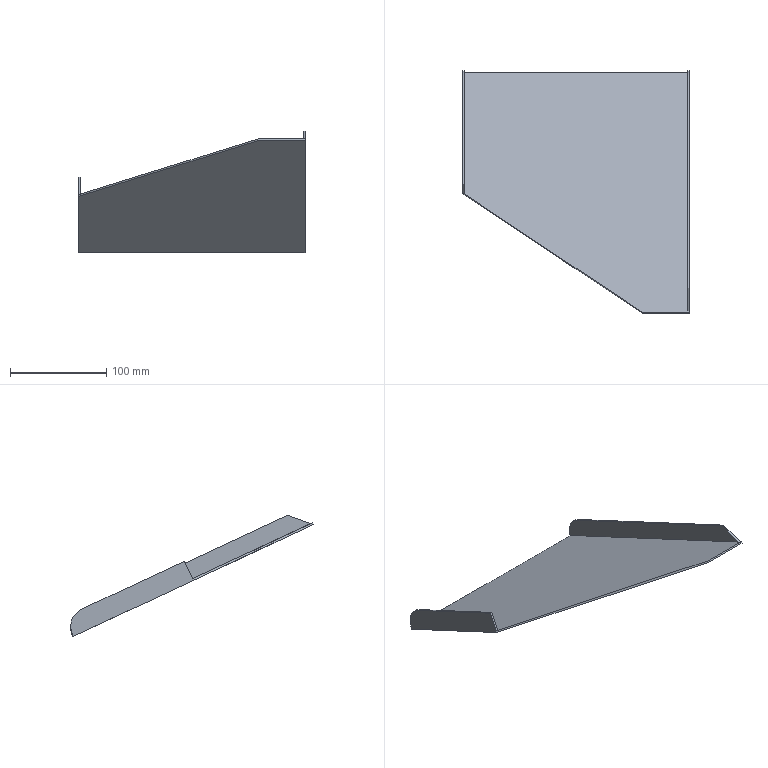Part | NX | features solid 2 | 1 solid | 15 faces | box 235.691 x 251.874 x 126.251 mm | volume 118871 mm3 | plane 13 | cylinder 2 | commonest cylinder face diameters 40 x2
STEP:
#1=CARTESIAN_POINT('',(530.986,470.,-185.082));
#2=VERTEX_POINT('',#1);
#3=CARTESIAN_POINT('',(344.309,594.452,-243.115));
#4=VERTEX_POINT('',#3);
#5=CARTESIAN_POINT('',(383.264,568.481,-231.004));
#6=DIRECTION('',(-0.8055,0.537,-0.2504));
#7=VECTOR('',#6,1000.);
#8=LINE('',#5,#7);
#9=EDGE_CURVE('',#2,#4,#8,.T.);
#10=ORIENTED_EDGE('',*,*,#9,.F.);
#11=CARTESIAN_POINT('',(530.986,470.845,-183.269));
#12=VERTEX_POINT('',#11);
#13=CARTESIAN_POINT('',(530.986,470.845,-183.269));
#14=DIRECTION('',(0.,-0.4226,-0.9063));
#15=VECTOR('',#14,1000.);
#16=LINE('',#13,#15);
#17=EDGE_CURVE('',#12,#2,#16,.T.);
#18=ORIENTED_EDGE('',*,*,#17,.F.);
#19=CARTESIAN_POINT('',(344.309,595.297,-241.302));
#20=VERTEX_POINT('',#19);
#21=CARTESIAN_POINT('',(383.264,569.326,-229.192));
#22=DIRECTION('',(-0.8055,0.537,-0.2504));
#23=VECTOR('',#22,1000.);
#24=LINE('',#21,#23);
#25=EDGE_CURVE('',#12,#20,#24,.T.);
#26=ORIENTED_EDGE('',*,*,#25,.T.);
#27=CARTESIAN_POINT('',(344.309,595.297,-241.302));
#28=DIRECTION('',(0.,-0.4226,-0.9063));
#29=VECTOR('',#28,1000.);
#30=LINE('',#27,#29);
#31=EDGE_CURVE('',#20,#4,#30,.T.);
#32=ORIENTED_EDGE('',*,*,#31,.T.);
#33=EDGE_LOOP('',(#10,#18,#26,#32));
#34=FACE_BOUND('',#33,.T.);
#35=CARTESIAN_POINT('',(383.264,569.326,-229.192));
#36=DIRECTION('',(-0.5925,-0.7301,0.3404));
#37=DIRECTION('',(0.7764,-0.6302,0.));
#38=AXIS2_PLACEMENT_3D('',#35,#36,#37);
#39=PLANE('',#38);
#40=ADVANCED_FACE('',(#34),#39,.T.);
#41=CARTESIAN_POINT('',(580.,470.,-185.082));
#42=VERTEX_POINT('',#41);
#43=CARTESIAN_POINT('',(570.,470.,-185.082));
#44=DIRECTION('',(-1.,0.,0.));
#45=VECTOR('',#44,1000.);
#46=LINE('',#43,#45);
#47=EDGE_CURVE('',#2,#42,#46,.F.);
#48=ORIENTED_EDGE('',*,*,#47,.T.);
#49=CARTESIAN_POINT('',(580.,470.845,-183.269));
#50=VERTEX_POINT('',#49);
#51=CARTESIAN_POINT('',(580.,470.845,-183.269));
#52=DIRECTION('',(0.,-0.4226,-0.9063));
#53=VECTOR('',#52,1000.);
#54=LINE('',#51,#53);
#55=EDGE_CURVE('',#50,#42,#54,.T.);
#56=ORIENTED_EDGE('',*,*,#55,.F.);
#57=CARTESIAN_POINT('',(570.,470.845,-183.269));
#58=DIRECTION('',(-1.,0.,0.));
#59=VECTOR('',#58,1000.);
#60=LINE('',#57,#59);
#61=EDGE_CURVE('',#12,#50,#60,.F.);
#62=ORIENTED_EDGE('',*,*,#61,.F.);
#63=ORIENTED_EDGE('',*,*,#17,.T.);
#64=EDGE_LOOP('',(#48,#56,#62,#63));
#65=FACE_BOUND('',#64,.T.);
#66=CARTESIAN_POINT('',(570.,470.845,-183.269));
#67=DIRECTION('',(0.,0.9063,-0.4226));
#68=DIRECTION('',(0.,0.4226,0.9063));
#69=AXIS2_PLACEMENT_3D('',#66,#67,#68);
#70=PLANE('',#69);
#71=ADVANCED_FACE('',(#65),#70,.F.);
#72=ORIENTED_EDGE('',*,*,#55,.T.);
#73=CARTESIAN_POINT('',(580.,720.,-301.659));
#74=VERTEX_POINT('',#73);
#75=CARTESIAN_POINT('',(580.,581.797,-237.214));
#76=DIRECTION('',(0.,-0.9063,0.4226));
#77=VECTOR('',#76,1000.);
#78=LINE('',#75,#77);
#79=EDGE_CURVE('',#74,#42,#78,.T.);
#80=ORIENTED_EDGE('',*,*,#79,.F.);
#81=CARTESIAN_POINT('',(580.,710.326,-275.08));
#82=VERTEX_POINT('',#81);
#83=CARTESIAN_POINT('',(580.,701.874,-293.206));
#84=DIRECTION('',(1.,0.,0.));
#85=DIRECTION('',(0.,0.,-1.));
#86=AXIS2_PLACEMENT_3D('',#83,#84,#85);
#87=CIRCLE('',#86,20.);
#88=EDGE_CURVE('',#74,#82,#87,.T.);
#89=ORIENTED_EDGE('',*,*,#88,.T.);
#90=CARTESIAN_POINT('',(580.,496.579,-175.408));
#91=VERTEX_POINT('',#90);
#92=CARTESIAN_POINT('',(580.,728.452,-283.533));
#93=DIRECTION('',(0.,-0.9063,0.4226));
#94=VECTOR('',#93,1000.);
#95=LINE('',#92,#94);
#96=EDGE_CURVE('',#82,#91,#95,.T.);
#97=ORIENTED_EDGE('',*,*,#96,.T.);
#98=CARTESIAN_POINT('',(580.,472.658,-184.114));
#99=VERTEX_POINT('',#98);
#100=CARTESIAN_POINT('',(580.,553.294,-154.765));
#101=DIRECTION('',(0.,-0.9397,-0.342));
#102=VECTOR('',#101,1000.);
#103=LINE('',#100,#102);
#104=EDGE_CURVE('',#91,#99,#103,.T.);
#105=ORIENTED_EDGE('',*,*,#104,.T.);
#106=CARTESIAN_POINT('',(580.,582.643,-235.401));
#107=DIRECTION('',(0.,-0.9063,0.4226));
#108=VECTOR('',#107,1000.);
#109=LINE('',#106,#108);
#110=EDGE_CURVE('',#99,#50,#109,.T.);
#111=ORIENTED_EDGE('',*,*,#110,.T.);
#112=EDGE_LOOP('',(#72,#80,#89,#97,#105,#111));
#113=FACE_BOUND('',#112,.T.);
#114=CARTESIAN_POINT('',(580.,582.643,-235.401));
#115=DIRECTION('',(1.,0.,0.));
#116=DIRECTION('',(0.,0.,-1.));
#117=AXIS2_PLACEMENT_3D('',#114,#115,#116);
#118=PLANE('',#117);
#119=ADVANCED_FACE('',(#113),#118,.T.);
#120=CARTESIAN_POINT('',(578.,720.,-301.659));
#121=VERTEX_POINT('',#120);
#122=CARTESIAN_POINT('',(578.,720.,-299.452));
#123=VERTEX_POINT('',#122);
#124=CARTESIAN_POINT('',(578.,720.,-430.));
#125=DIRECTION('',(0.,0.,-1.));
#126=VECTOR('',#125,1000.);
#127=LINE('',#124,#126);
#128=EDGE_CURVE('',#121,#123,#127,.F.);
#129=ORIENTED_EDGE('',*,*,#128,.F.);
#130=CARTESIAN_POINT('',(344.309,720.,-301.659));
#131=VERTEX_POINT('',#130);
#132=CARTESIAN_POINT('',(570.,720.,-301.659));
#133=DIRECTION('',(-1.,0.,0.));
#134=VECTOR('',#133,1000.);
#135=LINE('',#132,#134);
#136=EDGE_CURVE('',#131,#121,#135,.F.);
#137=ORIENTED_EDGE('',*,*,#136,.F.);
#138=CARTESIAN_POINT('',(344.309,720.,-299.452));
#139=VERTEX_POINT('',#138);
#140=CARTESIAN_POINT('',(344.309,720.,-430.));
#141=DIRECTION('',(0.,0.,1.));
#142=VECTOR('',#141,1000.);
#143=LINE('',#140,#142);
#144=EDGE_CURVE('',#139,#131,#143,.F.);
#145=ORIENTED_EDGE('',*,*,#144,.F.);
#146=CARTESIAN_POINT('',(346.309,720.,-299.452));
#147=VERTEX_POINT('',#146);
#148=CARTESIAN_POINT('',(570.,720.,-299.452));
#149=DIRECTION('',(-1.,0.,0.));
#150=VECTOR('',#149,1000.);
#151=LINE('',#148,#150);
#152=EDGE_CURVE('',#139,#147,#151,.F.);
#153=ORIENTED_EDGE('',*,*,#152,.T.);
#154=CARTESIAN_POINT('',(570.,720.,-299.452));
#155=DIRECTION('',(-1.,0.,0.));
#156=VECTOR('',#155,1000.);
#157=LINE('',#154,#156);
#158=EDGE_CURVE('',#147,#123,#157,.F.);
#159=ORIENTED_EDGE('',*,*,#158,.T.);
#160=EDGE_LOOP('',(#129,#137,#145,#153,#159));
#161=FACE_BOUND('',#160,.T.);
#162=CARTESIAN_POINT('',(188.564,720.,-430.));
#163=DIRECTION('',(0.,-1.,0.));
#164=DIRECTION('',(-1.,0.,0.));
#165=AXIS2_PLACEMENT_3D('',#162,#163,#164);
#166=PLANE('',#165);
#167=ADVANCED_FACE('',(#161),#166,.F.);
#168=CARTESIAN_POINT('',(344.309,524.315,-210.409));
#169=DIRECTION('',(0.,-0.9063,0.4226));
#170=VECTOR('',#169,1000.);
#171=LINE('',#168,#170);
#172=EDGE_CURVE('',#131,#4,#171,.T.);
#173=ORIENTED_EDGE('',*,*,#172,.T.);
#174=ORIENTED_EDGE('',*,*,#31,.F.);
#175=CARTESIAN_POINT('',(344.309,603.749,-223.176));
#176=VERTEX_POINT('',#175);
#177=CARTESIAN_POINT('',(344.309,595.297,-241.302));
#178=DIRECTION('',(0.,0.4226,0.9063));
#179=VECTOR('',#178,1000.);
#180=LINE('',#177,#179);
#181=EDGE_CURVE('',#20,#176,#180,.T.);
#182=ORIENTED_EDGE('',*,*,#181,.T.);
#183=CARTESIAN_POINT('',(344.309,710.326,-272.873));
#184=VERTEX_POINT('',#183);
#185=CARTESIAN_POINT('',(344.309,728.452,-281.326));
#186=DIRECTION('',(0.,-0.9063,0.4226));
#187=VECTOR('',#186,1000.);
#188=LINE('',#185,#187);
#189=EDGE_CURVE('',#184,#176,#188,.T.);
#190=ORIENTED_EDGE('',*,*,#189,.F.);
#191=CARTESIAN_POINT('',(344.309,701.874,-291.));
#192=DIRECTION('',(-1.,0.,0.));
#193=DIRECTION('',(0.,-1.,0.));
#194=AXIS2_PLACEMENT_3D('',#191,#192,#193);
#195=CIRCLE('',#194,20.);
#196=EDGE_CURVE('',#184,#139,#195,.T.);
#197=ORIENTED_EDGE('',*,*,#196,.T.);
#198=ORIENTED_EDGE('',*,*,#144,.T.);
#199=EDGE_LOOP('',(#173,#174,#182,#190,#197,#198));
#200=FACE_BOUND('',#199,.T.);
#201=CARTESIAN_POINT('',(344.309,525.16,-208.597));
#202=DIRECTION('',(1.,0.,0.));
#203=DIRECTION('',(0.,1.,0.));
#204=AXIS2_PLACEMENT_3D('',#201,#202,#203);
#205=PLANE('',#204);
#206=ADVANCED_FACE('',(#200),#205,.F.);
#207=CARTESIAN_POINT('',(578.,472.658,-184.114));
#208=VERTEX_POINT('',#207);
#209=CARTESIAN_POINT('',(570.,472.658,-184.114));
#210=DIRECTION('',(-1.,0.,0.));
#211=VECTOR('',#210,1000.);
#212=LINE('',#209,#211);
#213=EDGE_CURVE('',#99,#208,#212,.T.);
#214=ORIENTED_EDGE('',*,*,#213,.T.);
#215=CARTESIAN_POINT('',(578.,582.643,-235.401));
#216=DIRECTION('',(0.,0.9063,-0.4226));
#217=VECTOR('',#216,1000.);
#218=LINE('',#215,#217);
#219=EDGE_CURVE('',#208,#123,#218,.T.);
#220=ORIENTED_EDGE('',*,*,#219,.T.);
#221=ORIENTED_EDGE('',*,*,#158,.F.);
#222=CARTESIAN_POINT('',(346.309,595.297,-241.302));
#223=VERTEX_POINT('',#222);
#224=CARTESIAN_POINT('',(346.309,720.,-299.452));
#225=DIRECTION('',(0.,-0.9063,0.4226));
#226=VECTOR('',#225,1000.);
#227=LINE('',#224,#226);
#228=EDGE_CURVE('',#147,#223,#227,.T.);
#229=ORIENTED_EDGE('',*,*,#228,.T.);
#230=CARTESIAN_POINT('',(344.309,595.297,-241.302));
#231=DIRECTION('',(1.,0.,0.));
#232=VECTOR('',#231,1000.);
#233=LINE('',#230,#232);
#234=EDGE_CURVE('',#20,#223,#233,.T.);
#235=ORIENTED_EDGE('',*,*,#234,.F.);
#236=ORIENTED_EDGE('',*,*,#25,.F.);
#237=ORIENTED_EDGE('',*,*,#61,.T.);
#238=ORIENTED_EDGE('',*,*,#110,.F.);
#239=EDGE_LOOP('',(#214,#220,#221,#229,#235,#236,#237,#238));
#240=FACE_BOUND('',#239,.T.);
#241=CARTESIAN_POINT('',(570.,582.643,-235.401));
#242=DIRECTION('',(0.,-0.4226,-0.9063));
#243=DIRECTION('',(-1.,0.,0.));
#244=AXIS2_PLACEMENT_3D('',#241,#242,#243);
#245=PLANE('',#244);
#246=ADVANCED_FACE('',(#240),#245,.F.);
#247=ORIENTED_EDGE('',*,*,#136,.T.);
#248=CARTESIAN_POINT('',(570.,720.,-301.659));
#249=DIRECTION('',(1.,0.,0.));
#250=VECTOR('',#249,1000.);
#251=LINE('',#248,#250);
#252=EDGE_CURVE('',#74,#121,#251,.F.);
#253=ORIENTED_EDGE('',*,*,#252,.F.);
#254=ORIENTED_EDGE('',*,*,#79,.T.);
#255=ORIENTED_EDGE('',*,*,#47,.F.);
#256=ORIENTED_EDGE('',*,*,#9,.T.);
#257=ORIENTED_EDGE('',*,*,#172,.F.);
#258=EDGE_LOOP('',(#247,#253,#254,#255,#256,#257));
#259=FACE_BOUND('',#258,.T.);
#260=CARTESIAN_POINT('',(570.,581.797,-237.214));
#261=DIRECTION('',(0.,-0.4226,-0.9063));
#262=DIRECTION('',(-1.,0.,0.));
#263=AXIS2_PLACEMENT_3D('',#260,#261,#262);
#264=PLANE('',#263);
#265=ADVANCED_FACE('',(#259),#264,.T.);
#266=CARTESIAN_POINT('',(346.309,710.326,-272.873));
#267=VERTEX_POINT('',#266);
#268=CARTESIAN_POINT('',(346.309,603.749,-223.176));
#269=VERTEX_POINT('',#268);
#270=CARTESIAN_POINT('',(346.309,728.452,-281.326));
#271=DIRECTION('',(0.,-0.9063,0.4226));
#272=VECTOR('',#271,1000.);
#273=LINE('',#270,#272);
#274=EDGE_CURVE('',#267,#269,#273,.T.);
#275=ORIENTED_EDGE('',*,*,#274,.F.);
#276=CARTESIAN_POINT('',(344.309,710.326,-272.873));
#277=DIRECTION('',(-1.,0.,0.));
#278=VECTOR('',#277,1000.);
#279=LINE('',#276,#278);
#280=EDGE_CURVE('',#267,#184,#279,.T.);
#281=ORIENTED_EDGE('',*,*,#280,.T.);
#282=ORIENTED_EDGE('',*,*,#189,.T.);
#283=CARTESIAN_POINT('',(344.309,603.749,-223.176));
#284=DIRECTION('',(1.,0.,0.));
#285=VECTOR('',#284,1000.);
#286=LINE('',#283,#285);
#287=EDGE_CURVE('',#176,#269,#286,.T.);
#288=ORIENTED_EDGE('',*,*,#287,.T.);
#289=EDGE_LOOP('',(#275,#281,#282,#288));
#290=FACE_BOUND('',#289,.T.);
#291=CARTESIAN_POINT('',(344.309,728.452,-281.326));
#292=DIRECTION('',(0.,-0.4226,-0.9063));
#293=DIRECTION('',(0.,-0.9063,0.4226));
#294=AXIS2_PLACEMENT_3D('',#291,#292,#293);
#295=PLANE('',#294);
#296=ADVANCED_FACE('',(#290),#295,.F.);
#297=ORIENTED_EDGE('',*,*,#228,.F.);
#298=CARTESIAN_POINT('',(346.309,701.874,-291.));
#299=DIRECTION('',(-1.,0.,0.));
#300=DIRECTION('',(0.,-1.,0.));
#301=AXIS2_PLACEMENT_3D('',#298,#299,#300);
#302=CIRCLE('',#301,20.);
#303=EDGE_CURVE('',#147,#267,#302,.F.);
#304=ORIENTED_EDGE('',*,*,#303,.T.);
#305=ORIENTED_EDGE('',*,*,#274,.T.);
#306=CARTESIAN_POINT('',(346.309,595.297,-241.302));
#307=DIRECTION('',(0.,0.4226,0.9063));
#308=VECTOR('',#307,1000.);
#309=LINE('',#306,#308);
#310=EDGE_CURVE('',#223,#269,#309,.T.);
#311=ORIENTED_EDGE('',*,*,#310,.F.);
#312=EDGE_LOOP('',(#297,#304,#305,#311));
#313=FACE_BOUND('',#312,.T.);
#314=CARTESIAN_POINT('',(346.309,720.,-299.452));
#315=DIRECTION('',(-1.,0.,0.));
#316=DIRECTION('',(0.,-1.,0.));
#317=AXIS2_PLACEMENT_3D('',#314,#315,#316);
#318=PLANE('',#317);
#319=ADVANCED_FACE('',(#313),#318,.F.);
#320=ORIENTED_EDGE('',*,*,#181,.F.);
#321=ORIENTED_EDGE('',*,*,#234,.T.);
#322=ORIENTED_EDGE('',*,*,#310,.T.);
#323=ORIENTED_EDGE('',*,*,#287,.F.);
#324=EDGE_LOOP('',(#320,#321,#322,#323));
#325=FACE_BOUND('',#324,.T.);
#326=CARTESIAN_POINT('',(344.309,595.297,-241.302));
#327=DIRECTION('',(0.,-0.9063,0.4226));
#328=DIRECTION('',(0.,0.4226,0.9063));
#329=AXIS2_PLACEMENT_3D('',#326,#327,#328);
#330=PLANE('',#329);
#331=ADVANCED_FACE('',(#325),#330,.T.);
#332=ORIENTED_EDGE('',*,*,#196,.F.);
#333=ORIENTED_EDGE('',*,*,#280,.F.);
#334=ORIENTED_EDGE('',*,*,#303,.F.);
#335=ORIENTED_EDGE('',*,*,#152,.F.);
#336=EDGE_LOOP('',(#332,#333,#334,#335));
#337=FACE_BOUND('',#336,.T.);
#338=CARTESIAN_POINT('',(344.309,701.874,-291.));
#339=DIRECTION('',(1.,0.,0.));
#340=DIRECTION('',(0.,1.,0.));
#341=AXIS2_PLACEMENT_3D('',#338,#339,#340);
#342=CYLINDRICAL_SURFACE('',#341,20.);
#343=ADVANCED_FACE('',(#337),#342,.T.);
#344=ORIENTED_EDGE('',*,*,#213,.F.);
#345=ORIENTED_EDGE('',*,*,#104,.F.);
#346=CARTESIAN_POINT('',(578.,496.579,-175.408));
#347=VERTEX_POINT('',#346);
#348=CARTESIAN_POINT('',(570.,496.579,-175.408));
#349=DIRECTION('',(1.,0.,0.));
#350=VECTOR('',#349,1000.);
#351=LINE('',#348,#350);
#352=EDGE_CURVE('',#347,#91,#351,.T.);
#353=ORIENTED_EDGE('',*,*,#352,.F.);
#354=CARTESIAN_POINT('',(578.,653.288,-118.37));
#355=DIRECTION('',(0.,0.9397,0.342));
#356=VECTOR('',#355,1000.);
#357=LINE('',#354,#356);
#358=EDGE_CURVE('',#208,#347,#357,.T.);
#359=ORIENTED_EDGE('',*,*,#358,.F.);
#360=EDGE_LOOP('',(#344,#345,#353,#359));
#361=FACE_BOUND('',#360,.T.);
#362=CARTESIAN_POINT('',(570.,470.,-185.082));
#363=DIRECTION('',(0.,-0.342,0.9397));
#364=DIRECTION('',(0.,-0.9397,-0.342));
#365=AXIS2_PLACEMENT_3D('',#362,#363,#364);
#366=PLANE('',#365);
#367=ADVANCED_FACE('',(#361),#366,.T.);
#368=ORIENTED_EDGE('',*,*,#96,.F.);
#369=CARTESIAN_POINT('',(578.,710.326,-275.08));
#370=VERTEX_POINT('',#369);
#371=CARTESIAN_POINT('',(570.,710.326,-275.08));
#372=DIRECTION('',(-1.,0.,0.));
#373=VECTOR('',#372,1000.);
#374=LINE('',#371,#373);
#375=EDGE_CURVE('',#82,#370,#374,.T.);
#376=ORIENTED_EDGE('',*,*,#375,.T.);
#377=CARTESIAN_POINT('',(578.,728.452,-283.533));
#378=DIRECTION('',(0.,-0.9063,0.4226));
#379=VECTOR('',#378,1000.);
#380=LINE('',#377,#379);
#381=EDGE_CURVE('',#370,#347,#380,.T.);
#382=ORIENTED_EDGE('',*,*,#381,.T.);
#383=ORIENTED_EDGE('',*,*,#352,.T.);
#384=EDGE_LOOP('',(#368,#376,#382,#383));
#385=FACE_BOUND('',#384,.T.);
#386=CARTESIAN_POINT('',(570.,728.452,-283.533));
#387=DIRECTION('',(0.,-0.4226,-0.9063));
#388=DIRECTION('',(0.,-0.9063,0.4226));
#389=AXIS2_PLACEMENT_3D('',#386,#387,#388);
#390=PLANE('',#389);
#391=ADVANCED_FACE('',(#385),#390,.F.);
#392=CARTESIAN_POINT('',(578.,701.874,-293.206));
#393=DIRECTION('',(-1.,0.,0.));
#394=DIRECTION('',(0.,0.,1.));
#395=AXIS2_PLACEMENT_3D('',#392,#393,#394);
#396=CIRCLE('',#395,20.);
#397=EDGE_CURVE('',#370,#121,#396,.T.);
#398=ORIENTED_EDGE('',*,*,#397,.T.);
#399=ORIENTED_EDGE('',*,*,#128,.T.);
#400=ORIENTED_EDGE('',*,*,#219,.F.);
#401=ORIENTED_EDGE('',*,*,#358,.T.);
#402=ORIENTED_EDGE('',*,*,#381,.F.);
#403=EDGE_LOOP('',(#398,#399,#400,#401,#402));
#404=FACE_BOUND('',#403,.T.);
#405=CARTESIAN_POINT('',(578.,720.,-301.659));
#406=DIRECTION('',(-1.,0.,0.));
#407=DIRECTION('',(0.,0.,1.));
#408=AXIS2_PLACEMENT_3D('',#405,#406,#407);
#409=PLANE('',#408);
#410=ADVANCED_FACE('',(#404),#409,.T.);
#411=ORIENTED_EDGE('',*,*,#88,.F.);
#412=ORIENTED_EDGE('',*,*,#252,.T.);
#413=ORIENTED_EDGE('',*,*,#397,.F.);
#414=ORIENTED_EDGE('',*,*,#375,.F.);
#415=EDGE_LOOP('',(#411,#412,#413,#414));
#416=FACE_BOUND('',#415,.T.);
#417=CARTESIAN_POINT('',(570.,701.874,-293.206));
#418=DIRECTION('',(-1.,0.,0.));
#419=DIRECTION('',(0.,0.,1.));
#420=AXIS2_PLACEMENT_3D('',#417,#418,#419);
#421=CYLINDRICAL_SURFACE('',#420,20.);
#422=ADVANCED_FACE('',(#416),#421,.T.);
#423=CLOSED_SHELL('',(#40,#71,#119,#167,#206,#246,#265,#296,#319,#331,#343,#367,#391,#410,#422));
#424=MANIFOLD_SOLID_BREP('',#423);
#425=(LENGTH_UNIT()NAMED_UNIT(*)SI_UNIT(.MILLI.,.METRE.));
#426=UNCERTAINTY_MEASURE_WITH_UNIT(LENGTH_MEASURE(0.00001),#425,'','');
#427=(NAMED_UNIT(*)PLANE_ANGLE_UNIT()SI_UNIT($,.RADIAN.));
#428=(NAMED_UNIT(*)SI_UNIT($,.STERADIAN.)SOLID_ANGLE_UNIT());
#429=(GEOMETRIC_REPRESENTATION_CONTEXT(3)GLOBAL_UNCERTAINTY_ASSIGNED_CONTEXT((#426))GLOBAL_UNIT_ASSIGNED_CONTEXT((#425,#427,#428))REPRESENTATION_CONTEXT('',''));
#430=ADVANCED_BREP_SHAPE_REPRESENTATION('',(#424),#429);